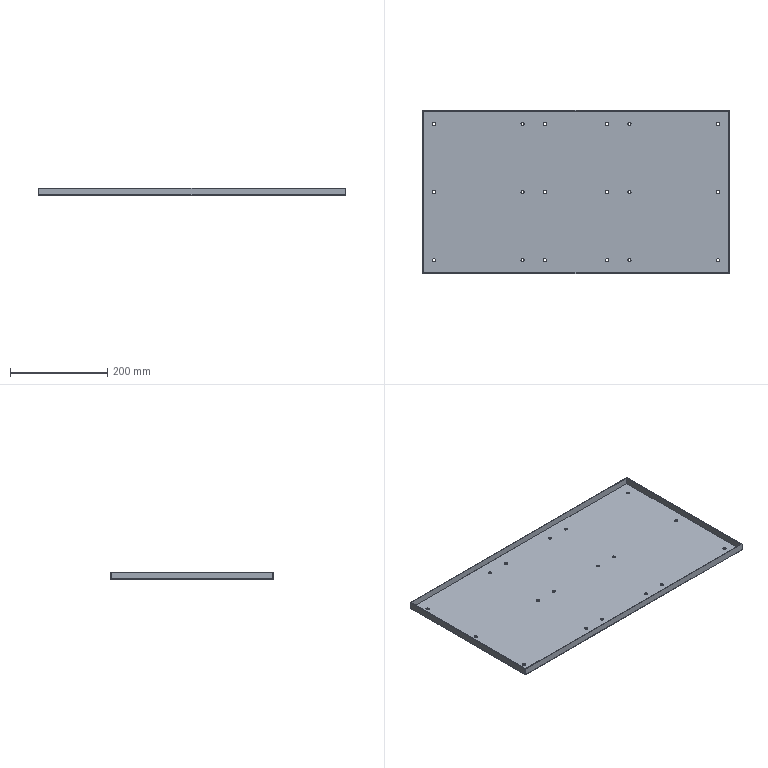Part | SolidWorks | features Extrusion 1, FlatPattern 1, FlattenBends 1, ICE 1, ProcessBends 1, Rip 1, SheetMetal 1, Shell 1 | 1 solid | 94 faces | box 630 x 336 x 15 mm | volume 354650 mm3 | plane 54 | cylinder 40 | commonest cylinder face diameters 6.5 x36 3 x4